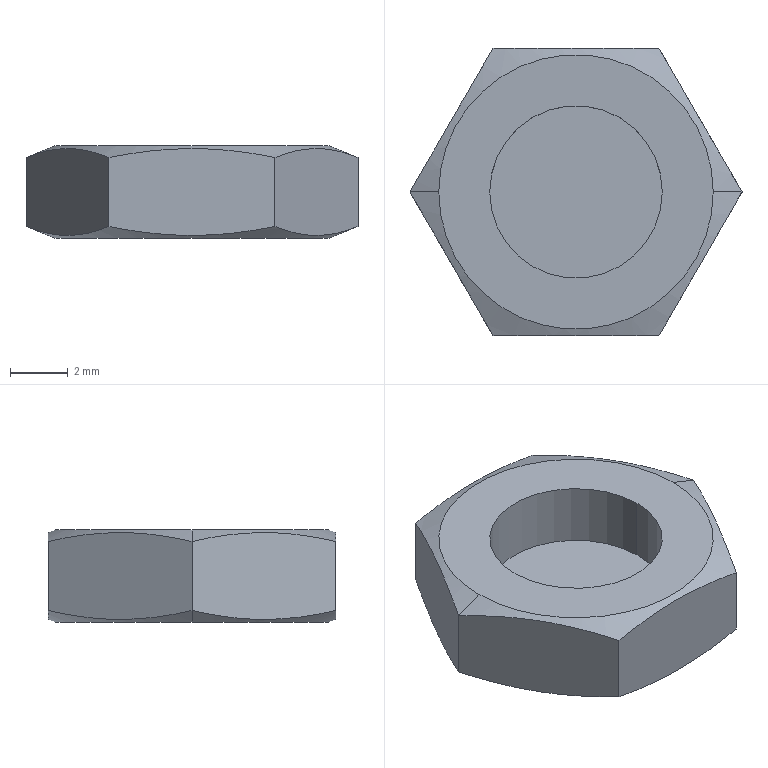Part | STEP file | JDC-75-5 | 1 solid | 15 faces | box 11.547 x 10 x 3.2 mm | volume 211.321 mm3 | plane 9 | cone 4 | cylinder 2 | commonest cylinder face diameters 6 x2